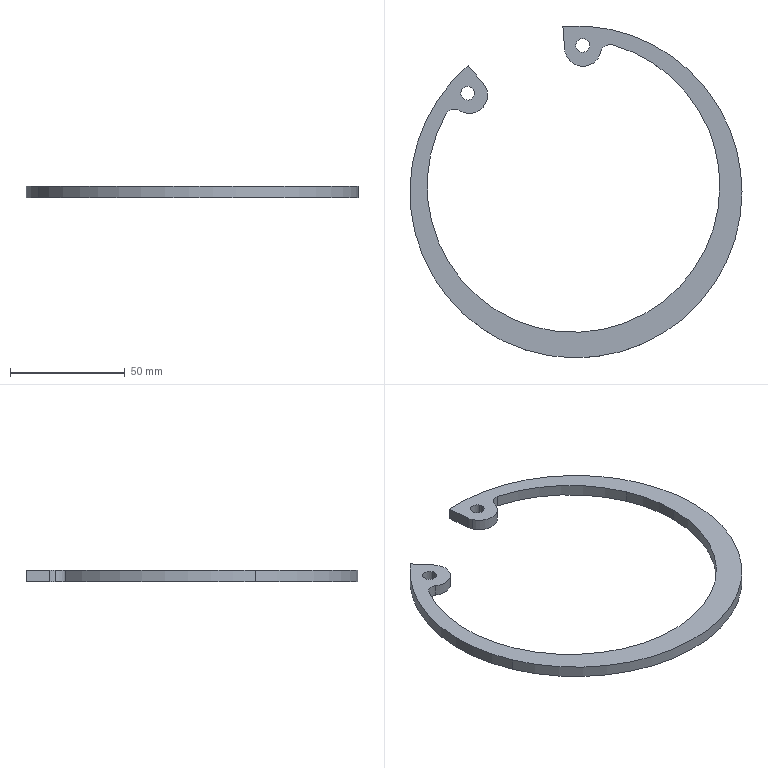Part | SolidWorks | features BaseBody 1 | 1 solid | 24 faces | box 145 x 145 x 5 mm | volume 18463 mm3 | cylinder 20 | plane 4 | commonest cylinder face diameters 6 x6 16 x4 127.8 x4 145 x4 8 x2
STEP:
#1=CARTESIAN_POINT('',(216.039,992.583,622.507));
#2=VERTEX_POINT('',#1);
#3=CARTESIAN_POINT('',(221.582,994.882,622.507));
#4=VERTEX_POINT('',#3);
#5=CARTESIAN_POINT('',(218.81,993.732,622.507));
#6=DIRECTION('',(0.,0.,-1.));
#7=DIRECTION('',(0.9237,0.383,0.));
#8=AXIS2_PLACEMENT_3D('',#5,#6,#7);
#9=CIRCLE('',#8,3.);
#10=EDGE_CURVE('',#2,#4,#9,.T.);
#11=ORIENTED_EDGE('',*,*,#10,.F.);
#12=CARTESIAN_POINT('',(221.81,993.732,622.507));
#13=VERTEX_POINT('',#12);
#14=CARTESIAN_POINT('',(218.81,993.732,622.507));
#15=DIRECTION('',(0.,0.,-1.));
#16=DIRECTION('',(0.9237,0.383,0.));
#17=AXIS2_PLACEMENT_3D('',#14,#15,#16);
#18=CIRCLE('',#17,3.);
#19=EDGE_CURVE('',#13,#2,#18,.T.);
#20=ORIENTED_EDGE('',*,*,#19,.F.);
#21=CARTESIAN_POINT('',(218.81,993.732,622.507));
#22=DIRECTION('',(0.,0.,-1.));
#23=DIRECTION('',(0.9237,0.383,0.));
#24=AXIS2_PLACEMENT_3D('',#21,#22,#23);
#25=CIRCLE('',#24,3.);
#26=EDGE_CURVE('',#4,#13,#25,.T.);
#27=ORIENTED_EDGE('',*,*,#26,.F.);
#28=EDGE_LOOP('',(#11,#20,#27));
#29=FACE_BOUND('',#28,.T.);
#30=CARTESIAN_POINT('',(266.346,1013.445,622.507));
#31=VERTEX_POINT('',#30);
#32=CARTESIAN_POINT('',(271.889,1015.743,622.507));
#33=VERTEX_POINT('',#32);
#34=CARTESIAN_POINT('',(269.117,1014.594,622.507));
#35=DIRECTION('',(0.,0.,-1.));
#36=DIRECTION('',(-0.9237,-0.383,0.));
#37=AXIS2_PLACEMENT_3D('',#34,#35,#36);
#38=CIRCLE('',#37,3.);
#39=EDGE_CURVE('',#31,#33,#38,.T.);
#40=ORIENTED_EDGE('',*,*,#39,.F.);
#41=CARTESIAN_POINT('',(272.117,1014.594,622.507));
#42=VERTEX_POINT('',#41);
#43=CARTESIAN_POINT('',(269.117,1014.594,622.507));
#44=DIRECTION('',(0.,0.,-1.));
#45=DIRECTION('',(-0.9237,-0.383,0.));
#46=AXIS2_PLACEMENT_3D('',#43,#44,#45);
#47=CIRCLE('',#46,3.);
#48=EDGE_CURVE('',#42,#31,#47,.T.);
#49=ORIENTED_EDGE('',*,*,#48,.F.);
#50=CARTESIAN_POINT('',(269.117,1014.594,622.507));
#51=DIRECTION('',(0.,0.,-1.));
#52=DIRECTION('',(-0.9237,-0.383,0.));
#53=AXIS2_PLACEMENT_3D('',#50,#51,#52);
#54=CIRCLE('',#53,3.);
#55=EDGE_CURVE('',#33,#42,#54,.T.);
#56=ORIENTED_EDGE('',*,*,#55,.F.);
#57=EDGE_LOOP('',(#40,#49,#56));
#58=FACE_BOUND('',#57,.T.);
#59=CARTESIAN_POINT('',(225.612,998.088,622.507));
#60=VERTEX_POINT('',#59);
#61=CARTESIAN_POINT('',(227.531,992.89,622.507));
#62=VERTEX_POINT('',#61);
#63=CARTESIAN_POINT('',(219.531,992.89,622.507));
#64=DIRECTION('',(0.,0.,-1.));
#65=DIRECTION('',(0.9237,0.383,0.));
#66=AXIS2_PLACEMENT_3D('',#63,#64,#65);
#67=CIRCLE('',#66,8.);
#68=EDGE_CURVE('',#60,#62,#67,.T.);
#69=ORIENTED_EDGE('',*,*,#68,.T.);
#70=CARTESIAN_POINT('',(215.17,986.182,622.507));
#71=VERTEX_POINT('',#70);
#72=CARTESIAN_POINT('',(219.531,992.89,622.507));
#73=DIRECTION('',(0.,0.,-1.));
#74=DIRECTION('',(0.9237,0.383,0.));
#75=AXIS2_PLACEMENT_3D('',#72,#73,#74);
#76=CIRCLE('',#75,8.);
#77=EDGE_CURVE('',#62,#71,#76,.T.);
#78=ORIENTED_EDGE('',*,*,#77,.T.);
#79=CARTESIAN_POINT('',(209.512,984.804,622.507));
#80=VERTEX_POINT('',#79);
#81=CARTESIAN_POINT('',(212.99,982.829,622.507));
#82=DIRECTION('',(0.,0.,1.));
#83=DIRECTION('',(-0.9237,-0.383,0.));
#84=AXIS2_PLACEMENT_3D('',#81,#82,#83);
#85=CIRCLE('',#84,4.);
#86=EDGE_CURVE('',#71,#80,#85,.T.);
#87=ORIENTED_EDGE('',*,*,#86,.T.);
#88=CARTESIAN_POINT('',(206.051,928.772,622.507));
#89=VERTEX_POINT('',#88);
#90=CARTESIAN_POINT('',(265.077,953.249,622.507));
#91=DIRECTION('',(0.,0.,1.));
#92=DIRECTION('',(0.9237,0.383,0.));
#93=AXIS2_PLACEMENT_3D('',#90,#91,#92);
#94=CIRCLE('',#93,63.9);
#95=EDGE_CURVE('',#80,#89,#94,.T.);
#96=ORIENTED_EDGE('',*,*,#95,.T.);
#97=CARTESIAN_POINT('',(328.977,953.249,622.507));
#98=VERTEX_POINT('',#97);
#99=CARTESIAN_POINT('',(265.077,953.249,622.507));
#100=DIRECTION('',(0.,0.,1.));
#101=DIRECTION('',(0.9237,0.383,0.));
#102=AXIS2_PLACEMENT_3D('',#99,#100,#101);
#103=CIRCLE('',#102,63.9);
#104=EDGE_CURVE('',#89,#98,#103,.T.);
#105=ORIENTED_EDGE('',*,*,#104,.T.);
#106=CARTESIAN_POINT('',(324.103,977.726,622.507));
#107=VERTEX_POINT('',#106);
#108=CARTESIAN_POINT('',(265.077,953.249,622.507));
#109=DIRECTION('',(0.,0.,1.));
#110=DIRECTION('',(0.9237,0.383,0.));
#111=AXIS2_PLACEMENT_3D('',#108,#109,#110);
#112=CIRCLE('',#111,63.9);
#113=EDGE_CURVE('',#98,#107,#112,.T.);
#114=ORIENTED_EDGE('',*,*,#113,.T.);
#115=CARTESIAN_POINT('',(282.006,1014.866,622.507));
#116=VERTEX_POINT('',#115);
#117=CARTESIAN_POINT('',(265.077,953.249,622.507));
#118=DIRECTION('',(0.,0.,1.));
#119=DIRECTION('',(0.9237,0.383,0.));
#120=AXIS2_PLACEMENT_3D('',#117,#118,#119);
#121=CIRCLE('',#120,63.9);
#122=EDGE_CURVE('',#107,#116,#121,.T.);
#123=ORIENTED_EDGE('',*,*,#122,.T.);
#124=CARTESIAN_POINT('',(277.032,1011.835,622.507));
#125=VERTEX_POINT('',#124);
#126=CARTESIAN_POINT('',(280.946,1011.009,622.507));
#127=DIRECTION('',(0.,0.,1.));
#128=DIRECTION('',(0.9237,0.383,0.));
#129=AXIS2_PLACEMENT_3D('',#126,#127,#128);
#130=CIRCLE('',#129,4.);
#131=EDGE_CURVE('',#116,#125,#130,.T.);
#132=ORIENTED_EDGE('',*,*,#131,.T.);
#133=CARTESIAN_POINT('',(261.815,1010.424,622.507));
#134=VERTEX_POINT('',#133);
#135=CARTESIAN_POINT('',(269.205,1013.488,622.507));
#136=DIRECTION('',(0.,0.,-1.));
#137=DIRECTION('',(-0.9237,-0.383,0.));
#138=AXIS2_PLACEMENT_3D('',#135,#136,#137);
#139=CIRCLE('',#138,8.);
#140=EDGE_CURVE('',#125,#134,#139,.T.);
#141=ORIENTED_EDGE('',*,*,#140,.T.);
#142=CARTESIAN_POINT('',(261.23,1012.857,622.507));
#143=VERTEX_POINT('',#142);
#144=CARTESIAN_POINT('',(269.205,1013.488,622.507));
#145=DIRECTION('',(0.,0.,-1.));
#146=DIRECTION('',(-0.9237,-0.383,0.));
#147=AXIS2_PLACEMENT_3D('',#144,#145,#146);
#148=CIRCLE('',#147,8.);
#149=EDGE_CURVE('',#134,#143,#148,.T.);
#150=ORIENTED_EDGE('',*,*,#149,.T.);
#151=CARTESIAN_POINT('',(260.433,1022.937,622.507));
#152=VERTEX_POINT('',#151);
#153=CARTESIAN_POINT('',(261.23,1012.857,622.507));
#154=DIRECTION('',(-0.07885,0.9969,0.));
#155=VECTOR('',#154,1000.);
#156=LINE('',#153,#155);
#157=EDGE_CURVE('',#143,#152,#156,.T.);
#158=ORIENTED_EDGE('',*,*,#157,.T.);
#159=CARTESIAN_POINT('',(333.12,978.434,622.507));
#160=VERTEX_POINT('',#159);
#161=CARTESIAN_POINT('',(266.149,950.663,622.507));
#162=DIRECTION('',(0.,0.,-1.));
#163=DIRECTION('',(0.9237,0.383,0.));
#164=AXIS2_PLACEMENT_3D('',#161,#162,#163);
#165=CIRCLE('',#164,72.5);
#166=EDGE_CURVE('',#152,#160,#165,.T.);
#167=ORIENTED_EDGE('',*,*,#166,.T.);
#168=CARTESIAN_POINT('',(338.649,950.663,622.507));
#169=VERTEX_POINT('',#168);
#170=CARTESIAN_POINT('',(266.149,950.663,622.507));
#171=DIRECTION('',(0.,0.,-1.));
#172=DIRECTION('',(0.9237,0.383,0.));
#173=AXIS2_PLACEMENT_3D('',#170,#171,#172);
#174=CIRCLE('',#173,72.5);
#175=EDGE_CURVE('',#160,#169,#174,.T.);
#176=ORIENTED_EDGE('',*,*,#175,.T.);
#177=CARTESIAN_POINT('',(199.179,922.891,622.507));
#178=VERTEX_POINT('',#177);
#179=CARTESIAN_POINT('',(266.149,950.663,622.507));
#180=DIRECTION('',(0.,0.,-1.));
#181=DIRECTION('',(0.9237,0.383,0.));
#182=AXIS2_PLACEMENT_3D('',#179,#180,#181);
#183=CIRCLE('',#182,72.5);
#184=EDGE_CURVE('',#169,#178,#183,.T.);
#185=ORIENTED_EDGE('',*,*,#184,.T.);
#186=CARTESIAN_POINT('',(219.043,1005.773,622.507));
#187=VERTEX_POINT('',#186);
#188=CARTESIAN_POINT('',(266.149,950.663,622.507));
#189=DIRECTION('',(0.,0.,-1.));
#190=DIRECTION('',(0.9237,0.383,0.));
#191=AXIS2_PLACEMENT_3D('',#188,#189,#190);
#192=CIRCLE('',#191,72.5);
#193=EDGE_CURVE('',#178,#187,#192,.T.);
#194=ORIENTED_EDGE('',*,*,#193,.T.);
#195=CARTESIAN_POINT('',(225.612,998.088,622.507));
#196=DIRECTION('',(0.6497,-0.7601,0.));
#197=VECTOR('',#196,1000.);
#198=LINE('',#195,#197);
#199=EDGE_CURVE('',#187,#60,#198,.T.);
#200=ORIENTED_EDGE('',*,*,#199,.T.);
#201=EDGE_LOOP('',(#69,#78,#87,#96,#105,#114,#123,#132,#141,#150,#158,#167,#176,#185,#194,#200));
#202=FACE_OUTER_BOUND('',#201,.T.);
#203=CARTESIAN_POINT('',(219.531,992.89,622.507));
#204=DIRECTION('',(0.,0.,1.));
#205=DIRECTION('',(1.,0.,0.));
#206=AXIS2_PLACEMENT_3D('',#203,#204,#205);
#207=PLANE('',#206);
#208=ADVANCED_FACE('',(#29,#58,#202),#207,.F.);
#209=CARTESIAN_POINT('',(272.117,1014.594,627.507));
#210=VERTEX_POINT('',#209);
#211=CARTESIAN_POINT('',(272.117,1014.594,627.507));
#212=DIRECTION('',(0.,0.,-1.));
#213=VECTOR('',#212,1000.);
#214=LINE('',#211,#213);
#215=EDGE_CURVE('',#210,#42,#214,.T.);
#216=ORIENTED_EDGE('',*,*,#215,.F.);
#217=CARTESIAN_POINT('',(271.889,1015.743,627.507));
#218=VERTEX_POINT('',#217);
#219=CARTESIAN_POINT('',(269.117,1014.594,627.507));
#220=DIRECTION('',(0.,0.,-1.));
#221=DIRECTION('',(-0.9237,-0.383,0.));
#222=AXIS2_PLACEMENT_3D('',#219,#220,#221);
#223=CIRCLE('',#222,3.);
#224=EDGE_CURVE('',#218,#210,#223,.T.);
#225=ORIENTED_EDGE('',*,*,#224,.F.);
#226=CARTESIAN_POINT('',(271.889,1015.743,627.507));
#227=DIRECTION('',(0.,0.,-1.));
#228=VECTOR('',#227,1000.);
#229=LINE('',#226,#228);
#230=EDGE_CURVE('',#218,#33,#229,.T.);
#231=ORIENTED_EDGE('',*,*,#230,.T.);
#232=ORIENTED_EDGE('',*,*,#55,.T.);
#233=EDGE_LOOP('',(#216,#225,#231,#232));
#234=FACE_OUTER_BOUND('',#233,.T.);
#235=CARTESIAN_POINT('',(269.117,1014.594,627.507));
#236=DIRECTION('',(0.,0.,-1.));
#237=DIRECTION('',(1.,0.,0.));
#238=AXIS2_PLACEMENT_3D('',#235,#236,#237);
#239=CYLINDRICAL_SURFACE('',#238,3.);
#240=ADVANCED_FACE('',(#234),#239,.F.);
#241=CARTESIAN_POINT('',(221.81,993.732,627.507));
#242=VERTEX_POINT('',#241);
#243=CARTESIAN_POINT('',(221.81,993.732,627.507));
#244=DIRECTION('',(0.,0.,-1.));
#245=VECTOR('',#244,1000.);
#246=LINE('',#243,#245);
#247=EDGE_CURVE('',#242,#13,#246,.T.);
#248=ORIENTED_EDGE('',*,*,#247,.F.);
#249=CARTESIAN_POINT('',(221.582,994.882,627.507));
#250=VERTEX_POINT('',#249);
#251=CARTESIAN_POINT('',(218.81,993.732,627.507));
#252=DIRECTION('',(0.,0.,-1.));
#253=DIRECTION('',(0.9237,0.383,0.));
#254=AXIS2_PLACEMENT_3D('',#251,#252,#253);
#255=CIRCLE('',#254,3.);
#256=EDGE_CURVE('',#250,#242,#255,.T.);
#257=ORIENTED_EDGE('',*,*,#256,.F.);
#258=CARTESIAN_POINT('',(221.582,994.882,627.507));
#259=DIRECTION('',(0.,0.,-1.));
#260=VECTOR('',#259,1000.);
#261=LINE('',#258,#260);
#262=EDGE_CURVE('',#250,#4,#261,.T.);
#263=ORIENTED_EDGE('',*,*,#262,.T.);
#264=ORIENTED_EDGE('',*,*,#26,.T.);
#265=EDGE_LOOP('',(#248,#257,#263,#264));
#266=FACE_OUTER_BOUND('',#265,.T.);
#267=CARTESIAN_POINT('',(218.81,993.732,627.507));
#268=DIRECTION('',(0.,0.,-1.));
#269=DIRECTION('',(1.,0.,0.));
#270=AXIS2_PLACEMENT_3D('',#267,#268,#269);
#271=CYLINDRICAL_SURFACE('',#270,3.);
#272=ADVANCED_FACE('',(#266),#271,.F.);
#273=CARTESIAN_POINT('',(219.043,1005.773,627.507));
#274=VERTEX_POINT('',#273);
#275=CARTESIAN_POINT('',(219.043,1005.773,627.507));
#276=DIRECTION('',(0.,0.,-1.));
#277=VECTOR('',#276,1000.);
#278=LINE('',#275,#277);
#279=EDGE_CURVE('',#274,#187,#278,.T.);
#280=ORIENTED_EDGE('',*,*,#279,.F.);
#281=CARTESIAN_POINT('',(225.612,998.088,627.507));
#282=VERTEX_POINT('',#281);
#283=CARTESIAN_POINT('',(225.612,998.088,627.507));
#284=DIRECTION('',(0.6497,-0.7601,0.));
#285=VECTOR('',#284,1000.);
#286=LINE('',#283,#285);
#287=EDGE_CURVE('',#274,#282,#286,.T.);
#288=ORIENTED_EDGE('',*,*,#287,.T.);
#289=CARTESIAN_POINT('',(225.612,998.088,627.507));
#290=DIRECTION('',(0.,0.,-1.));
#291=VECTOR('',#290,1000.);
#292=LINE('',#289,#291);
#293=EDGE_CURVE('',#282,#60,#292,.T.);
#294=ORIENTED_EDGE('',*,*,#293,.T.);
#295=ORIENTED_EDGE('',*,*,#199,.F.);
#296=EDGE_LOOP('',(#280,#288,#294,#295));
#297=FACE_OUTER_BOUND('',#296,.T.);
#298=CARTESIAN_POINT('',(225.612,998.088,627.507));
#299=DIRECTION('',(-0.7601,-0.6497,0.));
#300=DIRECTION('',(-0.6497,0.7601,0.));
#301=AXIS2_PLACEMENT_3D('',#298,#299,#300);
#302=PLANE('',#301);
#303=ADVANCED_FACE('',(#297),#302,.F.);
#304=CARTESIAN_POINT('',(333.12,978.434,627.507));
#305=VERTEX_POINT('',#304);
#306=CARTESIAN_POINT('',(333.12,978.434,627.507));
#307=DIRECTION('',(0.,0.,-1.));
#308=VECTOR('',#307,1000.);
#309=LINE('',#306,#308);
#310=EDGE_CURVE('',#305,#160,#309,.T.);
#311=ORIENTED_EDGE('',*,*,#310,.T.);
#312=ORIENTED_EDGE('',*,*,#166,.F.);
#313=CARTESIAN_POINT('',(260.433,1022.937,627.507));
#314=VERTEX_POINT('',#313);
#315=CARTESIAN_POINT('',(260.433,1022.937,627.507));
#316=DIRECTION('',(0.,0.,-1.));
#317=VECTOR('',#316,1000.);
#318=LINE('',#315,#317);
#319=EDGE_CURVE('',#314,#152,#318,.T.);
#320=ORIENTED_EDGE('',*,*,#319,.F.);
#321=CARTESIAN_POINT('',(266.149,950.663,627.507));
#322=DIRECTION('',(0.,0.,-1.));
#323=DIRECTION('',(0.9237,0.383,0.));
#324=AXIS2_PLACEMENT_3D('',#321,#322,#323);
#325=CIRCLE('',#324,72.5);
#326=EDGE_CURVE('',#314,#305,#325,.T.);
#327=ORIENTED_EDGE('',*,*,#326,.T.);
#328=EDGE_LOOP('',(#311,#312,#320,#327));
#329=FACE_OUTER_BOUND('',#328,.T.);
#330=CARTESIAN_POINT('',(266.149,950.663,627.507));
#331=DIRECTION('',(0.,0.,-1.));
#332=DIRECTION('',(1.,0.,0.));
#333=AXIS2_PLACEMENT_3D('',#330,#331,#332);
#334=CYLINDRICAL_SURFACE('',#333,72.5);
#335=ADVANCED_FACE('',(#329),#334,.T.);
#336=CARTESIAN_POINT('',(261.23,1012.857,627.507));
#337=VERTEX_POINT('',#336);
#338=CARTESIAN_POINT('',(261.23,1012.857,627.507));
#339=DIRECTION('',(0.,0.,-1.));
#340=VECTOR('',#339,1000.);
#341=LINE('',#338,#340);
#342=EDGE_CURVE('',#337,#143,#341,.T.);
#343=ORIENTED_EDGE('',*,*,#342,.F.);
#344=CARTESIAN_POINT('',(261.23,1012.857,627.507));
#345=DIRECTION('',(-0.07885,0.9969,0.));
#346=VECTOR('',#345,1000.);
#347=LINE('',#344,#346);
#348=EDGE_CURVE('',#337,#314,#347,.T.);
#349=ORIENTED_EDGE('',*,*,#348,.T.);
#350=ORIENTED_EDGE('',*,*,#319,.T.);
#351=ORIENTED_EDGE('',*,*,#157,.F.);
#352=EDGE_LOOP('',(#343,#349,#350,#351));
#353=FACE_OUTER_BOUND('',#352,.T.);
#354=CARTESIAN_POINT('',(261.23,1012.857,627.507));
#355=DIRECTION('',(0.9969,0.07885,0.));
#356=DIRECTION('',(0.,0.,-1.));
#357=AXIS2_PLACEMENT_3D('',#354,#355,#356);
#358=PLANE('',#357);
#359=ADVANCED_FACE('',(#353),#358,.F.);
#360=CARTESIAN_POINT('',(261.815,1010.424,627.507));
#361=VERTEX_POINT('',#360);
#362=CARTESIAN_POINT('',(261.815,1010.424,627.507));
#363=DIRECTION('',(0.,0.,-1.));
#364=VECTOR('',#363,1000.);
#365=LINE('',#362,#364);
#366=EDGE_CURVE('',#361,#134,#365,.T.);
#367=ORIENTED_EDGE('',*,*,#366,.T.);
#368=ORIENTED_EDGE('',*,*,#140,.F.);
#369=CARTESIAN_POINT('',(277.032,1011.835,627.507));
#370=VERTEX_POINT('',#369);
#371=CARTESIAN_POINT('',(277.032,1011.835,627.507));
#372=DIRECTION('',(0.,0.,-1.));
#373=VECTOR('',#372,1000.);
#374=LINE('',#371,#373);
#375=EDGE_CURVE('',#370,#125,#374,.T.);
#376=ORIENTED_EDGE('',*,*,#375,.F.);
#377=CARTESIAN_POINT('',(269.205,1013.488,627.507));
#378=DIRECTION('',(0.,0.,-1.));
#379=DIRECTION('',(-0.9237,-0.383,0.));
#380=AXIS2_PLACEMENT_3D('',#377,#378,#379);
#381=CIRCLE('',#380,8.);
#382=EDGE_CURVE('',#370,#361,#381,.T.);
#383=ORIENTED_EDGE('',*,*,#382,.T.);
#384=EDGE_LOOP('',(#367,#368,#376,#383));
#385=FACE_OUTER_BOUND('',#384,.T.);
#386=CARTESIAN_POINT('',(269.205,1013.488,627.507));
#387=DIRECTION('',(0.,0.,-1.));
#388=DIRECTION('',(1.,0.,0.));
#389=AXIS2_PLACEMENT_3D('',#386,#387,#388);
#390=CYLINDRICAL_SURFACE('',#389,8.);
#391=ADVANCED_FACE('',(#385),#390,.T.);
#392=CARTESIAN_POINT('',(282.006,1014.866,627.507));
#393=VERTEX_POINT('',#392);
#394=CARTESIAN_POINT('',(282.006,1014.866,627.507));
#395=DIRECTION('',(0.,0.,-1.));
#396=VECTOR('',#395,1000.);
#397=LINE('',#394,#396);
#398=EDGE_CURVE('',#393,#116,#397,.T.);
#399=ORIENTED_EDGE('',*,*,#398,.F.);
#400=CARTESIAN_POINT('',(280.946,1011.009,627.507));
#401=DIRECTION('',(0.,0.,1.));
#402=DIRECTION('',(0.9237,0.383,0.));
#403=AXIS2_PLACEMENT_3D('',#400,#401,#402);
#404=CIRCLE('',#403,4.);
#405=EDGE_CURVE('',#393,#370,#404,.T.);
#406=ORIENTED_EDGE('',*,*,#405,.T.);
#407=ORIENTED_EDGE('',*,*,#375,.T.);
#408=ORIENTED_EDGE('',*,*,#131,.F.);
#409=EDGE_LOOP('',(#399,#406,#407,#408));
#410=FACE_OUTER_BOUND('',#409,.T.);
#411=CARTESIAN_POINT('',(280.946,1011.009,627.507));
#412=DIRECTION('',(0.,0.,-1.));
#413=DIRECTION('',(1.,0.,0.));
#414=AXIS2_PLACEMENT_3D('',#411,#412,#413);
#415=CYLINDRICAL_SURFACE('',#414,4.);
#416=ADVANCED_FACE('',(#410),#415,.F.);
#417=CARTESIAN_POINT('',(206.051,928.772,627.507));
#418=VERTEX_POINT('',#417);
#419=CARTESIAN_POINT('',(206.051,928.772,627.507));
#420=DIRECTION('',(0.,0.,-1.));
#421=VECTOR('',#420,1000.);
#422=LINE('',#419,#421);
#423=EDGE_CURVE('',#418,#89,#422,.T.);
#424=ORIENTED_EDGE('',*,*,#423,.T.);
#425=ORIENTED_EDGE('',*,*,#95,.F.);
#426=CARTESIAN_POINT('',(209.512,984.804,627.507));
#427=VERTEX_POINT('',#426);
#428=CARTESIAN_POINT('',(209.512,984.804,627.507));
#429=DIRECTION('',(0.,0.,-1.));
#430=VECTOR('',#429,1000.);
#431=LINE('',#428,#430);
#432=EDGE_CURVE('',#427,#80,#431,.T.);
#433=ORIENTED_EDGE('',*,*,#432,.F.);
#434=CARTESIAN_POINT('',(265.077,953.249,627.507));
#435=DIRECTION('',(0.,0.,1.));
#436=DIRECTION('',(0.9237,0.383,0.));
#437=AXIS2_PLACEMENT_3D('',#434,#435,#436);
#438=CIRCLE('',#437,63.9);
#439=EDGE_CURVE('',#427,#418,#438,.T.);
#440=ORIENTED_EDGE('',*,*,#439,.T.);
#441=EDGE_LOOP('',(#424,#425,#433,#440));
#442=FACE_OUTER_BOUND('',#441,.T.);
#443=CARTESIAN_POINT('',(265.077,953.249,627.507));
#444=DIRECTION('',(0.,0.,-1.));
#445=DIRECTION('',(1.,0.,0.));
#446=AXIS2_PLACEMENT_3D('',#443,#444,#445);
#447=CYLINDRICAL_SURFACE('',#446,63.9);
#448=ADVANCED_FACE('',(#442),#447,.F.);
#449=CARTESIAN_POINT('',(215.17,986.182,627.507));
#450=VERTEX_POINT('',#449);
#451=CARTESIAN_POINT('',(215.17,986.182,627.507));
#452=DIRECTION('',(0.,0.,-1.));
#453=VECTOR('',#452,1000.);
#454=LINE('',#451,#453);
#455=EDGE_CURVE('',#450,#71,#454,.T.);
#456=ORIENTED_EDGE('',*,*,#455,.F.);
#457=CARTESIAN_POINT('',(212.99,982.829,627.507));
#458=DIRECTION('',(0.,0.,1.));
#459=DIRECTION('',(-0.9237,-0.383,0.));
#460=AXIS2_PLACEMENT_3D('',#457,#458,#459);
#461=CIRCLE('',#460,4.);
#462=EDGE_CURVE('',#450,#427,#461,.T.);
#463=ORIENTED_EDGE('',*,*,#462,.T.);
#464=ORIENTED_EDGE('',*,*,#432,.T.);
#465=ORIENTED_EDGE('',*,*,#86,.F.);
#466=EDGE_LOOP('',(#456,#463,#464,#465));
#467=FACE_OUTER_BOUND('',#466,.T.);
#468=CARTESIAN_POINT('',(212.99,982.829,627.507));
#469=DIRECTION('',(0.,0.,-1.));
#470=DIRECTION('',(1.,0.,0.));
#471=AXIS2_PLACEMENT_3D('',#468,#469,#470);
#472=CYLINDRICAL_SURFACE('',#471,4.);
#473=ADVANCED_FACE('',(#467),#472,.F.);
#474=CARTESIAN_POINT('',(227.531,992.89,627.507));
#475=VERTEX_POINT('',#474);
#476=CARTESIAN_POINT('',(227.531,992.89,627.507));
#477=DIRECTION('',(0.,0.,-1.));
#478=VECTOR('',#477,1000.);
#479=LINE('',#476,#478);
#480=EDGE_CURVE('',#475,#62,#479,.T.);
#481=ORIENTED_EDGE('',*,*,#480,.F.);
#482=CARTESIAN_POINT('',(219.531,992.89,627.507));
#483=DIRECTION('',(0.,0.,-1.));
#484=DIRECTION('',(0.9237,0.383,0.));
#485=AXIS2_PLACEMENT_3D('',#482,#483,#484);
#486=CIRCLE('',#485,8.);
#487=EDGE_CURVE('',#475,#450,#486,.T.);
#488=ORIENTED_EDGE('',*,*,#487,.T.);
#489=ORIENTED_EDGE('',*,*,#455,.T.);
#490=ORIENTED_EDGE('',*,*,#77,.F.);
#491=EDGE_LOOP('',(#481,#488,#489,#490));
#492=FACE_OUTER_BOUND('',#491,.T.);
#493=CARTESIAN_POINT('',(219.531,992.89,627.507));
#494=DIRECTION('',(0.,0.,-1.));
#495=DIRECTION('',(1.,0.,0.));
#496=AXIS2_PLACEMENT_3D('',#493,#494,#495);
#497=CYLINDRICAL_SURFACE('',#496,8.);
#498=ADVANCED_FACE('',(#492),#497,.T.);
#499=CARTESIAN_POINT('',(266.346,1013.445,627.507));
#500=VERTEX_POINT('',#499);
#501=CARTESIAN_POINT('',(269.117,1014.594,627.507));
#502=DIRECTION('',(0.,0.,-1.));
#503=DIRECTION('',(-0.9237,-0.383,0.));
#504=AXIS2_PLACEMENT_3D('',#501,#502,#503);
#505=CIRCLE('',#504,3.);
#506=EDGE_CURVE('',#500,#218,#505,.T.);
#507=ORIENTED_EDGE('',*,*,#506,.T.);
#508=ORIENTED_EDGE('',*,*,#224,.T.);
#509=CARTESIAN_POINT('',(269.117,1014.594,627.507));
#510=DIRECTION('',(0.,0.,-1.));
#511=DIRECTION('',(-0.9237,-0.383,0.));
#512=AXIS2_PLACEMENT_3D('',#509,#510,#511);
#513=CIRCLE('',#512,3.);
#514=EDGE_CURVE('',#210,#500,#513,.T.);
#515=ORIENTED_EDGE('',*,*,#514,.T.);
#516=EDGE_LOOP('',(#507,#508,#515));
#517=FACE_BOUND('',#516,.T.);
#518=CARTESIAN_POINT('',(216.039,992.583,627.507));
#519=VERTEX_POINT('',#518);
#520=CARTESIAN_POINT('',(218.81,993.732,627.507));
#521=DIRECTION('',(0.,0.,-1.));
#522=DIRECTION('',(0.9237,0.383,0.));
#523=AXIS2_PLACEMENT_3D('',#520,#521,#522);
#524=CIRCLE('',#523,3.);
#525=EDGE_CURVE('',#519,#250,#524,.T.);
#526=ORIENTED_EDGE('',*,*,#525,.T.);
#527=ORIENTED_EDGE('',*,*,#256,.T.);
#528=CARTESIAN_POINT('',(218.81,993.732,627.507));
#529=DIRECTION('',(0.,0.,-1.));
#530=DIRECTION('',(0.9237,0.383,0.));
#531=AXIS2_PLACEMENT_3D('',#528,#529,#530);
#532=CIRCLE('',#531,3.);
#533=EDGE_CURVE('',#242,#519,#532,.T.);
#534=ORIENTED_EDGE('',*,*,#533,.T.);
#535=EDGE_LOOP('',(#526,#527,#534));
#536=FACE_BOUND('',#535,.T.);
#537=CARTESIAN_POINT('',(219.531,992.89,627.507));
#538=DIRECTION('',(0.,0.,-1.));
#539=DIRECTION('',(0.9237,0.383,0.));
#540=AXIS2_PLACEMENT_3D('',#537,#538,#539);
#541=CIRCLE('',#540,8.);
#542=EDGE_CURVE('',#282,#475,#541,.T.);
#543=ORIENTED_EDGE('',*,*,#542,.F.);
#544=ORIENTED_EDGE('',*,*,#287,.F.);
#545=CARTESIAN_POINT('',(199.179,922.891,627.507));
#546=VERTEX_POINT('',#545);
#547=CARTESIAN_POINT('',(266.149,950.663,627.507));
#548=DIRECTION('',(0.,0.,-1.));
#549=DIRECTION('',(0.9237,0.383,0.));
#550=AXIS2_PLACEMENT_3D('',#547,#548,#549);
#551=CIRCLE('',#550,72.5);
#552=EDGE_CURVE('',#546,#274,#551,.T.);
#553=ORIENTED_EDGE('',*,*,#552,.F.);
#554=CARTESIAN_POINT('',(338.649,950.663,627.507));
#555=VERTEX_POINT('',#554);
#556=CARTESIAN_POINT('',(266.149,950.663,627.507));
#557=DIRECTION('',(0.,0.,-1.));
#558=DIRECTION('',(0.9237,0.383,0.));
#559=AXIS2_PLACEMENT_3D('',#556,#557,#558);
#560=CIRCLE('',#559,72.5);
#561=EDGE_CURVE('',#555,#546,#560,.T.);
#562=ORIENTED_EDGE('',*,*,#561,.F.);
#563=CARTESIAN_POINT('',(266.149,950.663,627.507));
#564=DIRECTION('',(0.,0.,-1.));
#565=DIRECTION('',(0.9237,0.383,0.));
#566=AXIS2_PLACEMENT_3D('',#563,#564,#565);
#567=CIRCLE('',#566,72.5);
#568=EDGE_CURVE('',#305,#555,#567,.T.);
#569=ORIENTED_EDGE('',*,*,#568,.F.);
#570=ORIENTED_EDGE('',*,*,#326,.F.);
#571=ORIENTED_EDGE('',*,*,#348,.F.);
#572=CARTESIAN_POINT('',(269.205,1013.488,627.507));
#573=DIRECTION('',(0.,0.,-1.));
#574=DIRECTION('',(-0.9237,-0.383,0.));
#575=AXIS2_PLACEMENT_3D('',#572,#573,#574);
#576=CIRCLE('',#575,8.);
#577=EDGE_CURVE('',#361,#337,#576,.T.);
#578=ORIENTED_EDGE('',*,*,#577,.F.);
#579=ORIENTED_EDGE('',*,*,#382,.F.);
#580=ORIENTED_EDGE('',*,*,#405,.F.);
#581=CARTESIAN_POINT('',(324.103,977.726,627.507));
#582=VERTEX_POINT('',#581);
#583=CARTESIAN_POINT('',(265.077,953.249,627.507));
#584=DIRECTION('',(0.,0.,1.));
#585=DIRECTION('',(0.9237,0.383,0.));
#586=AXIS2_PLACEMENT_3D('',#583,#584,#585);
#587=CIRCLE('',#586,63.9);
#588=EDGE_CURVE('',#582,#393,#587,.T.);
#589=ORIENTED_EDGE('',*,*,#588,.F.);
#590=CARTESIAN_POINT('',(328.977,953.249,627.507));
#591=VERTEX_POINT('',#590);
#592=CARTESIAN_POINT('',(265.077,953.249,627.507));
#593=DIRECTION('',(0.,0.,1.));
#594=DIRECTION('',(0.9237,0.383,0.));
#595=AXIS2_PLACEMENT_3D('',#592,#593,#594);
#596=CIRCLE('',#595,63.9);
#597=EDGE_CURVE('',#591,#582,#596,.T.);
#598=ORIENTED_EDGE('',*,*,#597,.F.);
#599=CARTESIAN_POINT('',(265.077,953.249,627.507));
#600=DIRECTION('',(0.,0.,1.));
#601=DIRECTION('',(0.9237,0.383,0.));
#602=AXIS2_PLACEMENT_3D('',#599,#600,#601);
#603=CIRCLE('',#602,63.9);
#604=EDGE_CURVE('',#418,#591,#603,.T.);
#605=ORIENTED_EDGE('',*,*,#604,.F.);
#606=ORIENTED_EDGE('',*,*,#439,.F.);
#607=ORIENTED_EDGE('',*,*,#462,.F.);
#608=ORIENTED_EDGE('',*,*,#487,.F.);
#609=EDGE_LOOP('',(#543,#544,#553,#562,#569,#570,#571,#578,#579,#580,#589,#598,#605,#606,#607,#608));
#610=FACE_OUTER_BOUND('',#609,.T.);
#611=CARTESIAN_POINT('',(219.531,992.89,627.507));
#612=DIRECTION('',(0.,0.,1.));
#613=DIRECTION('',(1.,0.,0.));
#614=AXIS2_PLACEMENT_3D('',#611,#612,#613);
#615=PLANE('',#614);
#616=ADVANCED_FACE('',(#517,#536,#610),#615,.T.);
#617=CARTESIAN_POINT('',(328.977,953.249,627.507));
#618=DIRECTION('',(0.,0.,-1.));
#619=VECTOR('',#618,1000.);
#620=LINE('',#617,#619);
#621=EDGE_CURVE('',#591,#98,#620,.T.);
#622=ORIENTED_EDGE('',*,*,#621,.F.);
#623=ORIENTED_EDGE('',*,*,#597,.T.);
#624=CARTESIAN_POINT('',(324.103,977.726,627.507));
#625=DIRECTION('',(0.,0.,-1.));
#626=VECTOR('',#625,1000.);
#627=LINE('',#624,#626);
#628=EDGE_CURVE('',#582,#107,#627,.T.);
#629=ORIENTED_EDGE('',*,*,#628,.T.);
#630=ORIENTED_EDGE('',*,*,#113,.F.);
#631=EDGE_LOOP('',(#622,#623,#629,#630));
#632=FACE_OUTER_BOUND('',#631,.T.);
#633=CARTESIAN_POINT('',(265.077,953.249,627.507));
#634=DIRECTION('',(0.,0.,-1.));
#635=DIRECTION('',(1.,0.,0.));
#636=AXIS2_PLACEMENT_3D('',#633,#634,#635);
#637=CYLINDRICAL_SURFACE('',#636,63.9);
#638=ADVANCED_FACE('',(#632),#637,.F.);
#639=ORIENTED_EDGE('',*,*,#588,.T.);
#640=ORIENTED_EDGE('',*,*,#398,.T.);
#641=ORIENTED_EDGE('',*,*,#122,.F.);
#642=ORIENTED_EDGE('',*,*,#628,.F.);
#643=EDGE_LOOP('',(#639,#640,#641,#642));
#644=FACE_OUTER_BOUND('',#643,.T.);
#645=CARTESIAN_POINT('',(265.077,953.249,627.507));
#646=DIRECTION('',(0.,0.,-1.));
#647=DIRECTION('',(1.,0.,0.));
#648=AXIS2_PLACEMENT_3D('',#645,#646,#647);
#649=CYLINDRICAL_SURFACE('',#648,63.9);
#650=ADVANCED_FACE('',(#644),#649,.F.);
#651=ORIENTED_EDGE('',*,*,#577,.T.);
#652=ORIENTED_EDGE('',*,*,#342,.T.);
#653=ORIENTED_EDGE('',*,*,#149,.F.);
#654=ORIENTED_EDGE('',*,*,#366,.F.);
#655=EDGE_LOOP('',(#651,#652,#653,#654));
#656=FACE_OUTER_BOUND('',#655,.T.);
#657=CARTESIAN_POINT('',(269.205,1013.488,627.507));
#658=DIRECTION('',(0.,0.,-1.));
#659=DIRECTION('',(1.,0.,0.));
#660=AXIS2_PLACEMENT_3D('',#657,#658,#659);
#661=CYLINDRICAL_SURFACE('',#660,8.);
#662=ADVANCED_FACE('',(#656),#661,.T.);
#663=ORIENTED_EDGE('',*,*,#552,.T.);
#664=ORIENTED_EDGE('',*,*,#279,.T.);
#665=ORIENTED_EDGE('',*,*,#193,.F.);
#666=CARTESIAN_POINT('',(199.179,922.891,627.507));
#667=DIRECTION('',(0.,0.,-1.));
#668=VECTOR('',#667,1000.);
#669=LINE('',#666,#668);
#670=EDGE_CURVE('',#546,#178,#669,.T.);
#671=ORIENTED_EDGE('',*,*,#670,.F.);
#672=EDGE_LOOP('',(#663,#664,#665,#671));
#673=FACE_OUTER_BOUND('',#672,.T.);
#674=CARTESIAN_POINT('',(266.149,950.663,627.507));
#675=DIRECTION('',(0.,0.,-1.));
#676=DIRECTION('',(1.,0.,0.));
#677=AXIS2_PLACEMENT_3D('',#674,#675,#676);
#678=CYLINDRICAL_SURFACE('',#677,72.5);
#679=ADVANCED_FACE('',(#673),#678,.T.);
#680=CARTESIAN_POINT('',(338.649,950.663,627.507));
#681=DIRECTION('',(0.,0.,-1.));
#682=VECTOR('',#681,1000.);
#683=LINE('',#680,#682);
#684=EDGE_CURVE('',#555,#169,#683,.T.);
#685=ORIENTED_EDGE('',*,*,#684,.F.);
#686=ORIENTED_EDGE('',*,*,#561,.T.);
#687=ORIENTED_EDGE('',*,*,#670,.T.);
#688=ORIENTED_EDGE('',*,*,#184,.F.);
#689=EDGE_LOOP('',(#685,#686,#687,#688));
#690=FACE_OUTER_BOUND('',#689,.T.);
#691=CARTESIAN_POINT('',(266.149,950.663,627.507));
#692=DIRECTION('',(0.,0.,-1.));
#693=DIRECTION('',(1.,0.,0.));
#694=AXIS2_PLACEMENT_3D('',#691,#692,#693);
#695=CYLINDRICAL_SURFACE('',#694,72.5);
#696=ADVANCED_FACE('',(#690),#695,.T.);
#697=ORIENTED_EDGE('',*,*,#525,.F.);
#698=CARTESIAN_POINT('',(216.039,992.583,627.507));
#699=DIRECTION('',(0.,0.,-1.));
#700=VECTOR('',#699,1000.);
#701=LINE('',#698,#700);
#702=EDGE_CURVE('',#519,#2,#701,.T.);
#703=ORIENTED_EDGE('',*,*,#702,.T.);
#704=ORIENTED_EDGE('',*,*,#10,.T.);
#705=ORIENTED_EDGE('',*,*,#262,.F.);
#706=EDGE_LOOP('',(#697,#703,#704,#705));
#707=FACE_OUTER_BOUND('',#706,.T.);
#708=CARTESIAN_POINT('',(218.81,993.732,627.507));
#709=DIRECTION('',(0.,0.,-1.));
#710=DIRECTION('',(1.,0.,0.));
#711=AXIS2_PLACEMENT_3D('',#708,#709,#710);
#712=CYLINDRICAL_SURFACE('',#711,3.);
#713=ADVANCED_FACE('',(#707),#712,.F.);
#714=ORIENTED_EDGE('',*,*,#506,.F.);
#715=CARTESIAN_POINT('',(266.346,1013.445,627.507));
#716=DIRECTION('',(0.,0.,-1.));
#717=VECTOR('',#716,1000.);
#718=LINE('',#715,#717);
#719=EDGE_CURVE('',#500,#31,#718,.T.);
#720=ORIENTED_EDGE('',*,*,#719,.T.);
#721=ORIENTED_EDGE('',*,*,#39,.T.);
#722=ORIENTED_EDGE('',*,*,#230,.F.);
#723=EDGE_LOOP('',(#714,#720,#721,#722));
#724=FACE_OUTER_BOUND('',#723,.T.);
#725=CARTESIAN_POINT('',(269.117,1014.594,627.507));
#726=DIRECTION('',(0.,0.,-1.));
#727=DIRECTION('',(1.,0.,0.));
#728=AXIS2_PLACEMENT_3D('',#725,#726,#727);
#729=CYLINDRICAL_SURFACE('',#728,3.);
#730=ADVANCED_FACE('',(#724),#729,.F.);
#731=ORIENTED_EDGE('',*,*,#568,.T.);
#732=ORIENTED_EDGE('',*,*,#684,.T.);
#733=ORIENTED_EDGE('',*,*,#175,.F.);
#734=ORIENTED_EDGE('',*,*,#310,.F.);
#735=EDGE_LOOP('',(#731,#732,#733,#734));
#736=FACE_OUTER_BOUND('',#735,.T.);
#737=CARTESIAN_POINT('',(266.149,950.663,627.507));
#738=DIRECTION('',(0.,0.,-1.));
#739=DIRECTION('',(1.,0.,0.));
#740=AXIS2_PLACEMENT_3D('',#737,#738,#739);
#741=CYLINDRICAL_SURFACE('',#740,72.5);
#742=ADVANCED_FACE('',(#736),#741,.T.);
#743=ORIENTED_EDGE('',*,*,#604,.T.);
#744=ORIENTED_EDGE('',*,*,#621,.T.);
#745=ORIENTED_EDGE('',*,*,#104,.F.);
#746=ORIENTED_EDGE('',*,*,#423,.F.);
#747=EDGE_LOOP('',(#743,#744,#745,#746));
#748=FACE_OUTER_BOUND('',#747,.T.);
#749=CARTESIAN_POINT('',(265.077,953.249,627.507));
#750=DIRECTION('',(0.,0.,-1.));
#751=DIRECTION('',(1.,0.,0.));
#752=AXIS2_PLACEMENT_3D('',#749,#750,#751);
#753=CYLINDRICAL_SURFACE('',#752,63.9);
#754=ADVANCED_FACE('',(#748),#753,.F.);
#755=ORIENTED_EDGE('',*,*,#542,.T.);
#756=ORIENTED_EDGE('',*,*,#480,.T.);
#757=ORIENTED_EDGE('',*,*,#68,.F.);
#758=ORIENTED_EDGE('',*,*,#293,.F.);
#759=EDGE_LOOP('',(#755,#756,#757,#758));
#760=FACE_OUTER_BOUND('',#759,.T.);
#761=CARTESIAN_POINT('',(219.531,992.89,627.507));
#762=DIRECTION('',(0.,0.,-1.));
#763=DIRECTION('',(1.,0.,0.));
#764=AXIS2_PLACEMENT_3D('',#761,#762,#763);
#765=CYLINDRICAL_SURFACE('',#764,8.);
#766=ADVANCED_FACE('',(#760),#765,.T.);
#767=ORIENTED_EDGE('',*,*,#533,.F.);
#768=ORIENTED_EDGE('',*,*,#247,.T.);
#769=ORIENTED_EDGE('',*,*,#19,.T.);
#770=ORIENTED_EDGE('',*,*,#702,.F.);
#771=EDGE_LOOP('',(#767,#768,#769,#770));
#772=FACE_OUTER_BOUND('',#771,.T.);
#773=CARTESIAN_POINT('',(218.81,993.732,627.507));
#774=DIRECTION('',(0.,0.,-1.));
#775=DIRECTION('',(1.,0.,0.));
#776=AXIS2_PLACEMENT_3D('',#773,#774,#775);
#777=CYLINDRICAL_SURFACE('',#776,3.);
#778=ADVANCED_FACE('',(#772),#777,.F.);
#779=ORIENTED_EDGE('',*,*,#514,.F.);
#780=ORIENTED_EDGE('',*,*,#215,.T.);
#781=ORIENTED_EDGE('',*,*,#48,.T.);
#782=ORIENTED_EDGE('',*,*,#719,.F.);
#783=EDGE_LOOP('',(#779,#780,#781,#782));
#784=FACE_OUTER_BOUND('',#783,.T.);
#785=CARTESIAN_POINT('',(269.117,1014.594,627.507));
#786=DIRECTION('',(0.,0.,-1.));
#787=DIRECTION('',(1.,0.,0.));
#788=AXIS2_PLACEMENT_3D('',#785,#786,#787);
#789=CYLINDRICAL_SURFACE('',#788,3.);
#790=ADVANCED_FACE('',(#784),#789,.F.);
#791=CLOSED_SHELL('',(#208,#240,#272,#303,#335,#359,#391,#416,#448,#473,#498,#616,#638,#650,#662,#679,#696,#713,#730,#742,#754,#766,#778,#790));
#792=MANIFOLD_SOLID_BREP('',#791);
#793=CARTESIAN_POINT('',(0.,0.,0.));
#794=DIRECTION('',(0.,0.,1.));
#795=DIRECTION('',(1.,0.,0.));
#796=AXIS2_PLACEMENT_3D('',#793,#794,#795);
#797=(LENGTH_UNIT()NAMED_UNIT(*)SI_UNIT(.MILLI.,.METRE.));
#798=UNCERTAINTY_MEASURE_WITH_UNIT(LENGTH_MEASURE(0.00001),#797,'','');
#799=(NAMED_UNIT(*)PLANE_ANGLE_UNIT()SI_UNIT($,.RADIAN.));
#800=(NAMED_UNIT(*)SI_UNIT($,.STERADIAN.)SOLID_ANGLE_UNIT());
#801=(GEOMETRIC_REPRESENTATION_CONTEXT(3)GLOBAL_UNCERTAINTY_ASSIGNED_CONTEXT((#798))GLOBAL_UNIT_ASSIGNED_CONTEXT((#797,#799,#800))REPRESENTATION_CONTEXT('',''));
#802=ADVANCED_BREP_SHAPE_REPRESENTATION('',(#792,#796),#801);